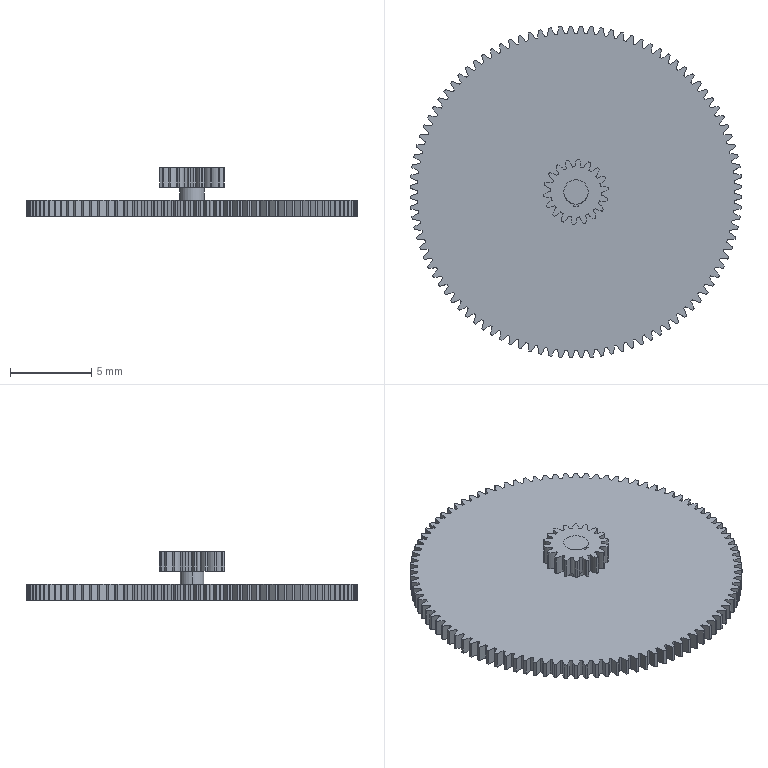Part | SolidWorks | 2 solids | 486 faces | box 20.395 x 20.395 x 3 mm | volume 326.572 mm3 | cylinder 242 | spline 236 | plane 8 | commonest cylinder face diameters 19.5 x101 20.4 x100 3.1 x18 4 x18 1.5 x5